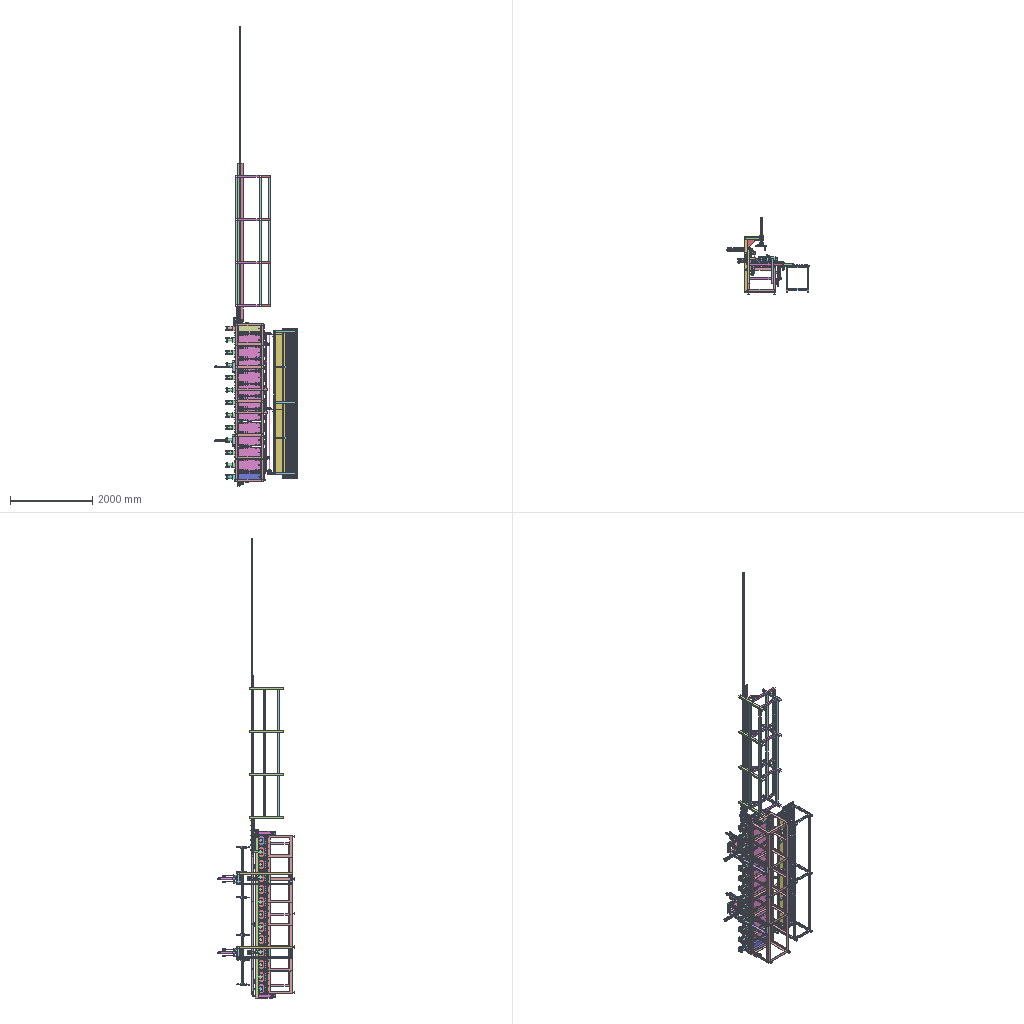Assembly | STEP file | 433 different items | 2728 placed | box 2000 x 1884 x 11210 mm
Parts list (item | name | quantity | parent item | size | volume), first 293 of 433 items:
1 | KHUNG SUON MAY DAP 3660 | x1 | in LAP KHUNG SUON MAY | 3868 x 784 x 600 mm | 15834108 mm3
2 | DIN 6915 M16 | x10 | in LAP KHUNG SUON MAY | 13 x 31.177 x 27 mm | 6064 mm3
3 | CHAN TANGDUA | x10 | in LAP KHUNG SUON MAY | 60 x 60 x 110 mm | 48381 mm3
4 | DIN 555 - replaced by DIN EN 24034 M16 | x8 | in LAP KHUNG SUON MAY | 13 x 27.713 x 24 mm | 4374 mm3
5 | DIN 6915 M12 | x52 | in LAP KHUNG SUON MAY | 10 x 25.403 x 22 mm | 3265 mm3
6 | MAT BAN CO LOGO 1_Welds | x1 | in MAT BAN CO LOGO 1 | 250 x 661.6 x 236 mm | 20450 mm3
7 | MAT BAN CO LOGO | x1 | in MAT BAN CO LOGO 1 | 250 x 633.6 x 80 mm | 6070480 mm3
8 | MAT TRUOT DAU BUA CO LOGO | x1 | in MAT BAN CO LOGO 1 | 250 x 300 x 24 mm | 1733556 mm3
9 | GA KHUON COI CO LOGO.dwg | x1 | in MAT BAN CO LOGO 1 | 250 x 186 x 260 mm | 3082669 mm3
10 | THANH CHINH NGAM TRUOT 2 | x2 | in MAT BAN CO LOGO 1 | 30 x 245 x 96 mm | 362252 mm3
11 | DAU BUA | x1 | in MAT BAN CO LOGO 1 | 130 x 95 x 200 mm | 1902985 mm3
12 | CHAN DO | x1 | in MAT BAN CO LOGO 1 | 250 x 55 x 70 mm | 565670 mm3
13 | CHAN DO2 | x1 | in MAT BAN CO LOGO 1 | 250 x 55 x 70 mm | 565670 mm3
14 | NGAM TRUOT | x1 | in MAT BAN CO LOGO 1 | 45 x 195 x 30 mm | 206561 mm3
15 | DIN 912 - replaced by DIN EN ISO 4762 M12 x 50 | x12 | in MAT BAN CO LOGO 1 | 62 x 18 x 18 mm | 8038 mm3
16 | DIN 912 - replaced by DIN EN ISO 4762 M14 x 40 | x9 | in MAT BAN CO LOGO 1 | 54 x 21 x 21 mm | 9880 mm3
17 | DIN 912 - replaced by DIN EN ISO 4762 M12 x 60 | x6 | in MAT BAN CO LOGO 1 | 72 x 18 x 18 mm | 9169 mm3
18 | DIN 912 - replaced by DIN EN ISO 4762 M10 x 50 | x6 | in MAT BAN CO LOGO 1 | 60 x 16 x 16 mm | 5580 mm3
19 | DIN 933 - replaced by DIN EN 24017 M10  x 40 | x4 | in MAT BAN CO LOGO 1 | 46.4 x 19.63 x 17 mm | 4638 mm3
20 | DIN 912 - replaced by DIN EN ISO 4762 M14 x 90 | x6 | in MAT BAN CO LOGO 1 | 104 x 21 x 21 mm | 17577 mm3
21 | MANG DAN PHOI CO LOGO | x1 | in MAT BAN CO LOGO 1 | 144 x 20 x 150 mm | 39222 mm3
22 | DIN 912 - replaced by DIN EN ISO 4762 M5 x 8 | x4 | in MAT BAN CO LOGO 1 | 13 x 8.5 x 8.5 mm | 395.808 mm3
23 | GA DAU NOI VAO DAU BUA | x1 | in MAT BAN CO LOGO 1 | 96 x 65 x 25 mm | 89450 mm3
24 | DAU NOI XY LANH 125 | x1 | in MAT BAN CO LOGO 1 | 56 x 56 x 39 mm | 36016 mm3
25 | Broached Socket Head Cap Screw - Metric M14x2 x 50 | x4 | in MAT BAN CO LOGO 1 | 64 x 21 x 21 mm | 11423 mm3
26 | giu lo xo day chot xien | x1 | in MAT BAN CO LOGO 1 | 80 x 25.5 x 50 mm | 77062 mm3
27 | Broached Socket Head Cap Screw - Metric M8x1.25 x 70 | x2 | in MAT BAN CO LOGO 1 | 78 x 13 x 13 mm | 4420 mm3
28 | Broached Hexagon Socket Set Screw - Flat Point - Metric M20x2.5 x 16 | x1 | in MAT BAN CO LOGO 1 | 16 x 20 x 20 mm | 3973 mm3
29 | Compress Spring1 | x1 | in Compress Spring | - | 1385 mm3
30 | TAM GA XYLANH GIUA | x1 | in MAT BAN CO LOGO 1 | 250 x 150 x 30 mm | 999493 mm3
31 | XYLANH _S_^80 | x1 | in MAT BAN CO LOGO 1 | 110 x 110 x 260 mm | 1251491 mm3
32 | PISTON XYLANH _S_^80 | x1 | in MAT BAN CO LOGO 1 | 40 x 40 x 118 mm | 134818 mm3
33 | TAN M35 BUOC 2 | x1 | in MAT BAN CO LOGO 1 | 57.735 x 50 x 14 mm | 16841 mm3
34 | NGAM TRUOT 2 | x1 | in MAT BAN CO LOGO 1 | 45 x 195 x 30 mm | 206561 mm3
35 | CHOT 14X100 | x4 | in MAT BAN CO LOGO 1 | 14 x 14 x 100 mm | 15235 mm3
36 | MIENG TRUNG GIAN DUOI | x1 | in KHUON AM CO LOGO | 250 x 135 x 24 mm | 656672 mm3
37 | KHUON BAO DUOI | x1 | in KHUON AM CO LOGO | 135 x 250 x 39.2 mm | 803564 mm3
38 | CHOT DINH VI 40 | x2 | in KHUON AM CO LOGO | 8 x 8 x 60 mm | 2993 mm3
39 | KHUON AM | x1 | in KHUON AM CO LOGO | 122.5 x 70 x 45.5 mm | 234393 mm3
40 | LOGO LOI | x1 | in KHUON AM CO LOGO | 22 x 16.4 x 40.3 mm | 10596 mm3
41 | LUOI GA TRON DUOI | x1 | in KHUON AM CO LOGO | 17 x 7 x 40.799 mm | 3679 mm3
42 | AS 1420 - Metric M8 x 25 | x6 | in KHUON AM CO LOGO | 33 x 13 x 13 mm | 2157 mm3
43 | AS 1420 - Metric M10 x 45 | x6 | in KHUON AM CO LOGO | 55 x 16 x 16 mm | 5187 mm3
44 | dao nhan khuon dap 3m6 | x1 | in KHUON AM CO LOGO | 45 x 34.3 x 57.1 mm | 58767 mm3
45 | con truot | x1 | in KHUON AM CO LOGO | 76 x 17 x 12 mm | 11883 mm3
46 | chot xien con truot | x1 | in KHUON AM CO LOGO | 15 x 47.7 x 30 mm | 18730 mm3
47 | cu dao nhan | x1 | in KHUON AM CO LOGO | 100 x 63 x 20 mm | 110399 mm3
48 | con chan chot xien | x1 | in KHUON AM CO LOGO | 20 x 10 x 18 mm | 1960 mm3
49 | Broached Socket Head Cap Screw - Metric M10x1.5 x 35 | x2 | in KHUON AM CO LOGO | 45 x 16 x 16 mm | 4403 mm3
50 | Broached Socket Head Cap Screw - Metric M10x1.5 x 50 | x1 | in KHUON AM CO LOGO | 60 x 16 x 16 mm | 5581 mm3
51 | Broached Socket Head Cap Screw - Metric M10x1.5 x 40 | x5 | in KHUON AM CO LOGO | 50 x 16 x 16 mm | 4795 mm3
52 | Broached Socket Head Cap Screw - Metric M6x1 x 16 | x1 | in KHUON AM CO LOGO | 22 x 10 x 10 mm | 839.144 mm3
53 | Broached Socket Head Cap Screw - Metric M10x1.5 x 30 | x1 | in KHUON AM CO LOGO | 40 x 16 x 16 mm | 4010 mm3
54 | luoi ga co logo | x1 | in KHUON AM CO LOGO | 10 x 15.6 x 51.124 mm | 6311 mm3
55 | Compress Spring1_2 | x1 | in Compress Spring_2 | - | 492.963 mm3
56 | Broached Socket Head Cap Screw - Metric M5x0.8 x 25 | x1 | in KHUON AM CO LOGO | 30 x 8.5 x 8.5 mm | 729.698 mm3
57 | BAT VOI MANG CA CO LOGO | x1 | in KHUON DUONG CO LOGO | 250 x 135 x 24 mm | 764464 mm3
58 | MIENG DE KHUON DUONG CO LOGO | x1 | in KHUON DUONG CO LOGO | 250 x 135 x 24 mm | 741333 mm3
59 | KHUON BAO TREN | x1 | in KHUON DUONG CO LOGO | 135 x 250 x 53 mm | 1111090 mm3
60 | CHOT DINH VI | x2 | in KHUON DUONG CO LOGO | 8 x 8 x 75 mm | 3747 mm3
61 | KHUON DUONG | x1 | in KHUON DUONG CO LOGO | 122.5 x 70 x 55.2 mm | 288291 mm3
62 | LUOI CAT | x1 | in KHUON DUONG CO LOGO | 88.8 x 70 x 40 mm | 196550 mm3
63 | LOGO LOM | x1 | in KHUON DUONG CO LOGO | 22 x 16.4 x 54.3 mm | 14617 mm3
64 | LUOI GA PHIA TREN | x1 | in KHUON DUONG CO LOGO | 17.5 x 11 x 53.3 mm | 9330 mm3
65 | LUOI GA TRON PHIA TREN | x1 | in KHUON DUONG CO LOGO | 17 x 7 x 57.44 mm | 5792 mm3
66 | THAN GA LUOI DOT | x1 | in KHUON DUONG CO LOGO | 14 x 22.5 x 77 mm | 19378 mm3
67 | LUOI DOT | x1 | in KHUON DUONG CO LOGO | 4 x 15.5 x 65.8 mm | 3850 mm3
68 | CHOT DUC 6.0 | x2 | in KHUON DUONG CO LOGO | 80 x 12.5 x 12.5 mm | 6322 mm3
69 | CHOT CAI | x1 | in KHUON DUONG CO LOGO | 6 x 6 x 22 mm | 620.89 mm3
70 | AS 1420 - Metric M8 x 30 | x1 | in KHUON DUONG CO LOGO | 38 x 13 x 13 mm | 2408 mm3
71 | AS 1420 - Metric M5 x 30 | x2 | in KHUON DUONG CO LOGO | 35 x 8.5 x 8.5 mm | 827.769 mm3
72 | AS 1420 - Metric M10 x 45_2 | x5 | in KHUON DUONG CO LOGO | 95 x 16 x 16 mm | 8328 mm3
73 | AS 1420 - Metric M8 x 55 | x1 | in KHUON DUONG CO LOGO | 63 x 13 x 13 mm | 3665 mm3
74 | CHOT TRUOT 6 LY | x4 | in KHUON DUONG CO LOGO | 6 x 6 x 8 mm | 225.049 mm3
75 | chot cam | x1 | in KHUON DUONG CO LOGO | 30 x 15 x 95 mm | 41659 mm3
76 | Broached Socket Head Cap Screw - Metric M10x1.5 x 80 | x5 | in KHUON DUONG CO LOGO | 90 x 16 x 16 mm | 7937 mm3
77 | Broached Socket Head Cap Screw - Metric M8x1.25 x 60 | x1 | in KHUON DUONG CO LOGO | 68 x 13 x 13 mm | 3917 mm3
78 | CHOT DAN DUONG | x4 | in KHUON DUONG CO LOGO | 18 x 18 x 95 mm | 15092 mm3
79 | Broached Socket Head Cap Screw - Metric M8x1.25 x 30 | x4 | in KHUON DUONG CO LOGO | 38 x 13 x 13 mm | 2409 mm3
80 | Broached Socket Head Cap Screw - Metric M5x0.8 x 25_2 | x2 | in KHUON DUONG CO LOGO | 30 x 8.5 x 8.5 mm | 729.698 mm3
81 | Broached Socket Head Cap Screw - Metric M12x1.75 x 30 | x4 | in KHUON DUONG CO LOGO | 42 x 18 x 18 mm | 5780 mm3
82 | noi khi | x1 | in KHUON DUONG CO LOGO | 37 x 27 x 14 mm | 4436 mm3
83 | MAT BAN KHONG LOGO_Welds | x1 | in 84 | 250 x 661.6 x 236 mm | 20450 mm3
84 | MAT BAN KHONG LOGO | x1 | in 84 | 250 x 633.6 x 80 mm | 6062488 mm3
85 | MAT TRUOT DAU BUA KHONG LOGO | x1 | in 84 | 250 x 300 x 24 mm | 1737062 mm3
86 | GA KHUON COI KHONG LOGO | x1 | in 84 | 250 x 186 x 203 mm | 2822642 mm3
87 | NGAM TRUOT_2 | x1 | in 84 | 45 x 195 x 30 mm | 206561 mm3
88 | THANH CHINH NGAM TRUOT 2_2 | x2 | in 84 | 30 x 245 x 96 mm | 362252 mm3
89 | CHAN DO_2 | x1 | in 84 | 250 x 55 x 70 mm | 565670 mm3
90 | DAU BUA_2 | x1 | in 84 | 130 x 95 x 200 mm | 1902822 mm3
91 | CHAN DO2_2 | x1 | in 84 | 250 x 55 x 70 mm | 565670 mm3
92 | DIN 912 - replaced by DIN EN ISO 4762 M14 x 35 | x7 | in 84 | 49 x 21 x 21 mm | 9111 mm3
93 | DIN 912 - replaced by DIN EN ISO 4762 M12 x 50_2 | x10 | in 84 | 62 x 18 x 18 mm | 8038 mm3
94 | DIN 912 - replaced by DIN EN ISO 4762 M14 x 50 | x4 | in 84 | 64 x 21 x 21 mm | 11420 mm3
95 | DIN 912 - replaced by DIN EN ISO 4762 M10 x 50_2 | x6 | in 84 | 60 x 16 x 16 mm | 5580 mm3
96 | DIN 933 - replaced by DIN EN 24017 M10  x 40_2 | x4 | in 84 | 46.4 x 19.63 x 17 mm | 4638 mm3
97 | DIN 912 - replaced by DIN EN ISO 4762 M10 x 40 | x4 | in 84 | 50 x 16 x 16 mm | 4794 mm3
98 | DIN 912 - replaced by DIN EN ISO 4762 M12 x 60_2 | x4 | in 84 | 72 x 18 x 18 mm | 9169 mm3
99 | DIN 912 - replaced by DIN EN ISO 4762 M12 x 70 | x4 | in 84 | 82 x 18 x 18 mm | 10300 mm3
100 | DIN 912 - replaced by DIN EN ISO 4762 M14 x 40_2 | x2 | in 84 | 54 x 21 x 21 mm | 9880 mm3
101 | DIN 912 - replaced by DIN EN ISO 4762 M14 x 90_2 | x6 | in 84 | 104 x 21 x 21 mm | 17577 mm3
102 | MANG DAN PHOI KHONG LOGO | x1 | in 84 | 144 x 20 x 150 mm | 39222 mm3
103 | DIN 912 - replaced by DIN EN ISO 4762 M5 x 8_2 | x4 | in 84 | 13 x 8.5 x 8.5 mm | 395.808 mm3
104 | CHOT 14X100_2 | x4 | in 84 | 14 x 14 x 100 mm | 15235 mm3
105 | NGAM TRUOT 2_2 | x1 | in 84 | 45 x 195 x 30 mm | 206561 mm3
106 | GA DAU NOI VAO DAU BUA_2 | x1 | in 84 | 96 x 65 x 25 mm | 89450 mm3
107 | PISTON XYLANH _S_^80_2 | x1 | in 84 | 40 x 40 x 118 mm | 134818 mm3
108 | XYLANH _S_^80_2 | x1 | in 84 | 110 x 110 x 260 mm | 1251491 mm3
109 | TAM GA XYLANH GIUA_2 | x1 | in 84 | 250 x 150 x 30 mm | 999493 mm3
110 | DAU NOI XY LANH 80 2 DAU NGAM | x1 | in 84 | 56 x 56 x 39 mm | 36016 mm3
111 | MIENG DE KHUON AM KO LOGO | x1 | in KHUON AM KHONG LOGO | 250 x 135 x 24 mm | 675291 mm3
112 | KHUON BAO DUOI_2 | x1 | in KHUON AM KHONG LOGO | 135 x 250 x 39.2 mm | 811850 mm3
113 | KHUON AM_2 | x1 | in KHUON AM KHONG LOGO | 122.5 x 70 x 45.5 mm | 246860 mm3
114 | LUOI GA PHIA DUOI | x1 | in KHUON AM KHONG LOGO | 17.5 x 11 x 39 mm | 7111 mm3
115 | LUOI GA TRON PHIA DUOI | x1 | in KHUON AM KHONG LOGO | 17 x 7 x 42.5 mm | 4171 mm3
116 | AS 1420 - Metric M5 x 30_2 | x2 | in KHUON AM KHONG LOGO | 35 x 8.5 x 8.5 mm | 827.769 mm3
117 | AS 1420 - Metric M8 x 25_2 | x3 | in KHUON AM KHONG LOGO | 33 x 13 x 13 mm | 2157 mm3
118 | AS 1420 - Metric M10 x 50 | x5 | in KHUON AM KHONG LOGO | 60 x 16 x 16 mm | 5580 mm3
119 | CHOT DINH VI 40_2 | x2 | in KHUON AM KHONG LOGO | 8 x 8 x 60 mm | 2993 mm3
120 | cu dao nhan khong logo | x1 | in KHUON AM KHONG LOGO | 110 x 63 x 20 mm | 127794 mm3
121 | Broached Socket Head Cap Screw - Metric M10x1.5 x 50_2 | x5 | in KHUON AM KHONG LOGO | 60 x 16 x 16 mm | 5581 mm3
122 | Broached Socket Head Cap Screw - Metric M10x1.5 x 40_2 | x1 | in KHUON AM KHONG LOGO | 50 x 16 x 16 mm | 4795 mm3
123 | Broached Socket Head Cap Screw - Metric M10x1.5 x 30_2 | x1 | in KHUON AM KHONG LOGO | 40 x 16 x 16 mm | 4010 mm3
124 | Broached Socket Head Cap Screw - Metric M8x1.25 x 30_2 | x4 | in KHUON AM KHONG LOGO | 38 x 13 x 13 mm | 2409 mm3
125 | Broached Socket Head Cap Screw - Metric M5x0.8 x 25_3 | x2 | in KHUON AM KHONG LOGO | 30 x 8.5 x 8.5 mm | 729.698 mm3
126 | Broached Socket Head Cap Screw - Metric M8x1.25 x 40 | x1 | in KHUON AM KHONG LOGO | 48 x 13 x 13 mm | 2912 mm3
127 | Broached Socket Head Cap Screw - Metric M10x1.5 x 35_2 | x2 | in KHUON AM KHONG LOGO | 45 x 16 x 16 mm | 4403 mm3
128 | Compress Spring1_3 | x1 | in Compress Spring_3 | - | 492.963 mm3
129 | dao nhan khong logo | x1 | in KHUON AM KHONG LOGO | 38 x 36 x 57.1 mm | 51330 mm3
130 | BAT VOI MANG CA KO LOGO | x1 | in KHUON DUONG KHONG LOGO | 250 x 135 x 24 mm | 764621 mm3
131 | MIENG DE KHUON DUONG KO LOGO | x1 | in KHUON DUONG KHONG LOGO | 250 x 135 x 24 mm | 743044 mm3
132 | EES - 2C 12x100 | x1 | in KHUON DUONG KHONG LOGO | 18 x 18 x 80 mm | 12722 mm3
133 | KHUON BAO TREN_2 | x1 | in KHUON DUONG KHONG LOGO | 135 x 250 x 53 mm | 1110961 mm3
134 | CHOT DINH VI_2 | x2 | in KHUON DUONG KHONG LOGO | 8 x 8 x 70 mm | 3496 mm3
135 | KHUON DUONG_2 | x1 | in KHUON DUONG KHONG LOGO | 122.5 x 70 x 55 mm | 306755 mm3
136 | LUOI CAT KHONG LOGO | x1 | in KHUON DUONG KHONG LOGO | 88.8 x 70 x 40 mm | 196221 mm3
137 | LUOI GA PHAI TREN | x1 | in KHUON DUONG KHONG LOGO | 10 x 15.6 x 59.05 mm | 8567 mm3
138 | LUOI GA TRON TREN | x1 | in KHUON DUONG KHONG LOGO | 17 x 7 x 55.799 mm | 5306 mm3
139 | CHOT CAI_2 | x1 | in KHUON DUONG KHONG LOGO | 6 x 6 x 22 mm | 620.89 mm3
140 | CHOT DUC 6.0_2 | x2 | in KHUON DUONG KHONG LOGO | 80 x 12.5 x 12.5 mm | 6322 mm3
141 | LUOI DOT_2 | x1 | in KHUON DUONG KHONG LOGO | 4 x 15.5 x 65.8 mm | 3850 mm3
142 | THAN GA LUOI DOT_2 | x1 | in KHUON DUONG KHONG LOGO | 14 x 22.5 x 77 mm | 19378 mm3
143 | AS 1420 - Metric M8 x 30_2 | x3 | in KHUON DUONG KHONG LOGO | 68 x 13 x 13 mm | 3916 mm3
144 | AS 1420 - Metric M5 x 30_3 | x2 | in KHUON DUONG KHONG LOGO | 35 x 8.5 x 8.5 mm | 827.769 mm3
145 | EES - 2C 12x100_2 | x3 | in KHUON DUONG KHONG LOGO | 18 x 18 x 100 mm | 15801 mm3
146 | AS 1420 - Metric M10 x 45_3 | x1 | in KHUON DUONG KHONG LOGO | 95 x 16 x 16 mm | 8328 mm3
147 | Compress Spring1_4 | x1 | in Compress Spring_4 | - | 3363 mm3
148 | CHOT TRUOT 6 LY_2 | x4 | in KHUON DUONG KHONG LOGO | 6 x 6 x 8 mm | 225.049 mm3
149 | chot cam_2 | x1 | in KHUON DUONG KHONG LOGO | 30 x 15 x 95 mm | 41659 mm3
150 | Broached Socket Head Cap Screw - Metric M8x1.25 x 30_3 | x1 | in KHUON DUONG KHONG LOGO | 38 x 13 x 13 mm | 2409 mm3
151 | Broached Socket Head Cap Screw - Metric M10x1.5 x 80_2 | x5 | in KHUON DUONG KHONG LOGO | 90 x 16 x 16 mm | 7937 mm3
152 | noi khi_2 | x1 | in KHUON DUONG KHONG LOGO | 37 x 27 x 14 mm | 4436 mm3
153 | MAT BAN GIUA_Welds | x11 | in 154 | 270 x 661.6 x 216 mm | 46200 mm3
154 | MAT BAN GIUA | x11 | in 154 | 270 x 633.6 x 80 mm | 5694476 mm3
155 | TAM TRUOT DAU BUA GIUA | x11 | in 154 | 270 x 300 x 24 mm | 1881062 mm3
156 | GA KHUON COI GIUA.dwg | x11 | in 154 | 270 x 166 x 203 mm | 2828600 mm3
157 | NGAM TRUOT_3 | x11 | in 154 | 45 x 194 x 30 mm | 205453 mm3
158 | THANH CHINH NGAM TRUOT 2_3 | x22 | in 154 | 30 x 294 x 96 mm | 428402 mm3
159 | DAU BUA_3 | x11 | in 154 | 130 x 95 x 200 mm | 1901919 mm3
160 | DIN 912 - replaced by DIN EN ISO 4762 M10 x 50_3 | x66 | in 154 | 60 x 16 x 16 mm | 5580 mm3
161 | DIN 912 - replaced by DIN EN ISO 4762 M14 x 35_2 | x99 | in 154 | 49 x 21 x 21 mm | 9111 mm3
162 | CHAN DO MAT BAN GIUA | x11 | in 154 | 270 x 55 x 70 mm | 612670 mm3
163 | CHAN DO MAT BAN GIUA BEN COI | x11 | in 154 | 270 x 55 x 70 mm | 612670 mm3
164 | DIN 912 - replaced by DIN EN ISO 4762 M12 x 50_3 | x110 | in 154 | 62 x 18 x 18 mm | 8038 mm3
165 | DIN 912 - replaced by DIN EN ISO 4762 M12 x 60_3 | x44 | in 154 | 72 x 18 x 18 mm | 9169 mm3
166 | DIN 912 - replaced by DIN EN ISO 4762 M12 x 70_2 | x44 | in 154 | 82 x 18 x 18 mm | 10300 mm3
167 | DIN 960 - replaced by DIN EN 28765 M10 x 1.25 x 40 | x44 | in 154 | 46.4 x 19.63 x 17 mm | 4694 mm3
168 | DIN 912 - replaced by DIN EN ISO 4762 M14 x 90_3 | x66 | in 154 | 104 x 21 x 21 mm | 17577 mm3
169 | MANG DAN PHOI BO GIUA | x11 | in 154 | 164 x 20 x 150 mm | 43722 mm3
170 | DIN 912 - replaced by DIN EN ISO 4762 M5 x 8_3 | x44 | in 154 | 13 x 8.5 x 8.5 mm | 395.808 mm3
171 | XYLANH _S_^80_3 | x11 | in 154 | 110 x 110 x 260 mm | 1251491 mm3
172 | TAM GA XYLANH GIUA_3 | x11 | in 154 | 250 x 150 x 30 mm | 1040750 mm3
173 | PISTON XYLANH _S_^80_3 | x11 | in 154 | 40 x 40 x 118 mm | 134818 mm3
174 | TAN M35 BUOC 2_2 | x11 | in 154 | 57.735 x 50 x 14 mm | 16841 mm3
175 | GA DAU NOI VAO DAU BUA_3 | x11 | in 154 | 96 x 65 x 25 mm | 89450 mm3
176 | DAU NOI BUA GIUA | x11 | in 154 | 76.5 x 56 x 56 mm | 107628 mm3
177 | BAC XAC DINH VI TRI XYLANH 80 | x11 | in 154 | 55 x 55 x 4 mm | 5655 mm3
178 | Broached Socket Head Cap Screw - Metric M14x2 x 50_2 | x44 | in 154 | 64 x 21 x 21 mm | 11423 mm3
179 | Broached Socket Head Cap Screw - Metric M10x1.5 x 45 | x44 | in 154 | 55 x 16 x 16 mm | 5188 mm3
180 | NGAM TRUOT 2_3 | x11 | in 154 | 45 x 194 x 30 mm | 205453 mm3
181 | CHOT 14X100_3 | x44 | in 154 | 14 x 14 x 100 mm | 15235 mm3
182 | TAM DE COI | x11 | in KHUON AM GIUA | 270 x 100 x 39 mm | 987341 mm3
183 | TAM COI | x11 | in KHUON AM GIUA | 270 x 68 x 25 mm | 392735 mm3
184 | DIN EN 22338 A - withdrawn 8 m6 x 40 - A | x22 | in KHUON AM GIUA | 40 x 8 x 8 mm | 1978 mm3
185 | DIN 912 - replaced by DIN EN ISO 4762 M8 x 50 | x66 | in KHUON AM GIUA | 58 x 13 x 13 mm | 3414 mm3
186 | TAM DE CHAY | x11 | in KHUON DUONG GIUA | 270 x 100 x 30 mm | 752474 mm3
187 | TAM LOT CHAY | x11 | in KHUON DUONG GIUA | 270 x 100 x 15 mm | 381434 mm3
188 | TAM GA CHAY | x11 | in KHUON DUONG GIUA | 270 x 100 x 30 mm | 706425 mm3
189 | COT DAN HUONG14X73 | x22 | in KHUON DUONG GIUA | 18 x 18 x 73 mm | 11705 mm3
190 | CHAY 6X10X50.dwg | x44 | in KHUON DUONG GIUA | 50 x 13 x 13 mm | 3399 mm3
191 | TAM CHAN PHOI | x11 | in KHUON DUONG GIUA | 270 x 24 x 12 mm | 71324 mm3
192 | DIN 912 - replaced by DIN EN ISO 4762 M12 x 40 | x44 | in KHUON DUONG GIUA | 52 x 18 x 18 mm | 6908 mm3
193 | DIN 912 - replaced by DIN EN ISO 4762 M8 x 30 | x44 | in KHUON DUONG GIUA | 38 x 13 x 13 mm | 2408 mm3
194 | DIN 912 - replaced by DIN EN ISO 4762 M8 x 60 | x66 | in KHUON DUONG GIUA | 68 x 13 x 13 mm | 3916 mm3
195 | BULONG BAC M8X10X56 | x22 | in KHUON DUONG GIUA | 15 x 15 x 74 mm | 6196 mm3
196 | bac 10.5-28 | x22 | in KHUON DUONG GIUA | 28 x 28 x 8 mm | 4233 mm3
197 | CU AN TOAN 10.4-20 - 5.5 | x22 | in KHUON DUONG GIUA | 30 x 30 x 5.5 mm | 1797 mm3
198 | LO XO D20d3X36 | x22 | in KHUON DUONG GIUA | 20.006 x 39.001 x 20.006 mm | 2345 mm3
199 | BULONG BAC M8X10X38 | x22 | in KHUON DUONG GIUA | 15 x 15 x 58 mm | 4939 mm3
200 | Compress Spring1_5 | x22 | in Compress Spring_5 | - | 1934 mm3
201 | CHAY 3.9 | x22 | in KHUON DUONG GIUA | 4 x 15.5 x 50 mm | 2874 mm3
202 | CHOT DINH VI 4X10 | x22 | in KHUON DUONG GIUA | 4 x 4 x 10 mm | 120.876 mm3
203 | Thanh T chinh 3m6 | x11 | in Automatic feeder punching | 24 x 37.5 x 3660 mm | 442294 mm3
204 | BCC3 H11_1B | x1 | in BCC3 H11B | 60 x 60 x 3440 mm | 1915667 mm3
205 | BCC3 H11_2B | x3 | in BCC3 H11B | 80 x 40 x 45 mm | 55899 mm3
206 | BCC3 H11_3 | x8 | in BCC3 H11B, BCC3 H12B, BCC3 H11_2 | 20 x 20 x 50 mm | 15708 mm3
207 | BCC3 H12_7B | x1 | in 207 | 40 x 75 x 4068 mm | 2791952 mm3
208 | BCC3 H12_8B | x2 | in 207 | 40 x 100 x 340 mm | 276708 mm3
209 | BCC3 H12_13 | x2 | in 207 | 70 x 68 x 10 mm | 46465 mm3
210 | Bulong M10_2.5F | x39 | in BCC3 G02B Motion1, BCC3 G03B Motion1, Automatic feeder punching | 18.475 x 16 x 31.5 mm | 3390 mm3
211 | Tan M10 | x23 | in BCC3 G02B Motion1, Automatic feeder punching, 237 | 18.475 x 16 x 9 mm | 1288 mm3
212 | BCC3 H11_5 | x10 | in BCC3 G02B Motion1, 237 | 15 x 15 x 1 mm | 90.124 mm3
213 | 6800ZZ | x7 | in BCC3 G02B Motion1 | 19 x 19 x 5 mm | 1015 mm3
214 | BCC3 H11_4 | x10 | in BCC3 G02B Motion1, 237 | 14 x 14 x 27 mm | 2265 mm3
215 | BCC3 H13_1 | x2 | in BCC3 G03B Motion1 | 290 x 22 x 100 mm | 496185 mm3
216 | - | x2 | - | 491 x 50.3 x 52 mm | 426363 mm3
217 | - | x6 | in BCC3 G03B Motion1, BCC3 G03B Motion2 | 471 x 40 x 40 mm | 111313 mm3
218 | 201100_M42x1_5_HI | x2 | - | 53.666 x 53.666 x 12 mm | 11002 mm3
219 | Bac truot | x4 | in BCC3 G03B Motion1 | 60 x 60 x 80 mm | 114067 mm3
220 | BCC3 H13_8B | x2 | in BCC3 H13_6B | 40 x 75 x 475 mm | 326568 mm3
221 | BCC3 H13_8B | x2 | in BCC3 H13_6B | 40 x 75 x 475 mm | 326568 mm3
222 | BCC3 H13_7 | x4 | in BCC3 H13_6B | 40 x 75 x 210 mm | 145356 mm3
223 | BCC3 H13_6 | x2 | in BCC3 H13_6B | 40 x 75 x 1270 mm | 877986 mm3
224 | BCC3 H13_6 | x2 | in BCC3 H13_6B | 40 x 75 x 1270 mm | 877986 mm3
225 | BCC3 H13_7 | x2 | in BCC3 H13_6B | 40 x 75 x 210 mm | 144819 mm3
226 | BCC3 H13_9B | x4 | in BCC3 H13_6B | 200 x 200 x 6 mm | 120000 mm3
227 | BCC3 H13_7 | x2 | in BCC3 H13_6B | 40 x 75 x 210 mm | 144819 mm3
228 | BCC3 H13_10 | x4 | in BCC3 H13_6B | 40 x 75 x 6 mm | 16643 mm3
229 | BCC3 H14_3B | x2 | in BCC3 H14B2_HI | 57 x 274 x 60 mm | 86752 mm3
230 | BCC3 H14_6B | x8 | in BCC3 H14B2_HI | 45 x 100 x 6 mm | 13452 mm3
231 | BCC3 H14_7 | x2 | in BCC3 H14B2_HI | 40 x 40 x 120 mm | 112909 mm3
232 | - | x2 | - | 50 x 50 x 517 mm | 322395 mm3
233 | - | x4 | in Automatic feeder punching | 32 x 32 x 503.2 mm | 60225 mm3
234 | - | x8 | in BCC3 G05 Motion1, Automatic feeder punching | 17 x 5 x 19.63 mm | 939.625 mm3
235 | BCC3 H16_1 | x3 | in 235 | 500 x 80 x 6 mm | 213344 mm3
236 | BCC3 H16_4 | x3 | in 235 | 32 x 16 x 32 mm | 8049 mm3
237 | BCC3 H16_7 | x3 | in 235 | 55 x 55 x 40 mm | 65270 mm3
238 | BCC3 H16_15 | x3 | in 235 | 20 x 20 x 230 mm | 17480 mm3
239 | BCC3 H16_5 | x3 | in BCC3 G05_1 | 25 x 25 x 8 mm | 1414 mm3
240 | BCC3 H16_2 | x3 | in BCC3 G05_1 | 95 x 10 x 95 mm | 53732 mm3
241 | BCC3 H16_6 | x3 | in BCC3 G05_1 | 30 x 30 x 2 mm | 1313 mm3
242 | Bulong M6_1.5F | x7 | in BCC3 G05_1, BCC3 G03B Motion2 | 11.547 x 10 x 19 mm | 768.3 mm3
243 | BCC3 H16_3 | x3 | in BCC3 G05_1 | 95 x 30 x 95 mm | 74080 mm3
244 | BCC3 H16_9 | x3 | in BCC3 G05_1 | 55 x 55 x 12 mm | 13803 mm3
245 | BCC3 H16_10 | x3 | in BCC3 G05_1 | 499.144 x 99.144 x 8 mm | 58375 mm3
246 | Bulong M8_2.5F | x6 | in BCC3 G05_1 | 12.73 x 14.699 x 30.15 mm | 1976 mm3
247 | BCC3 H16_8 | x1 | in BCC3 G05_2 | 25 x 25 x 3385 mm | 2110006 mm3
248 | BCC3 H16_11 | x4 | in BCC3 G05 Motion1, BCC3 H14B1_HI | 20 x 550 x 20 mm | 172727 mm3
249 | BCC3 H16_12 | x2 | in BCC3 G05 Motion1 | 83 x 40 x 30 mm | 84627 mm3
250 | BCC3 H16_13 | x1 | in BCC3 G05 Motion1 | 20 x 20 x 3390 mm | 1063554 mm3
251 | Gear motor - 12V (6 holes)_Default | x1 | in BCC3 G05 Motion1 | 124.05 x 100.1 x 199.5 mm | 340663 mm3
252 | BCC3 H16_14 | x1 | in BCC3 G05 Motion1 | 120 x 80 x 15 mm | 111656 mm3
253 | BCC3 H16_16 | x3 | in BCC3 G05 Motion1 | 5 x 5 x 30 mm | 750 mm3
254 | Bulong M8_2F | x8 | in BCC3 G05 Motion1, Automatic feeder punching | 12.73 x 14.699 x 25.15 mm | 1725 mm3
255 | - | x4 | in BCC3 G05 Motion1 | 32 x 32 x 303.2 mm | 37606 mm3
256 | BCC3 H17_1 | x2 | in BCC3 H17_HI | 130 x 120 x 60 mm | 136586 mm3
257 | BCC3 H17_2 | x2 | in BCC3 H17_HI | 40 x 40 x 150 mm | 141183 mm3
258 | BCC3 H17_3 | x4 | in BCC3 H17_HI | 120 x 90 x 6 mm | 32400 mm3
259 | - | x2 | - | 50 x 50 x 317 mm | 245584 mm3
260 | BCC3 H12_1B | x1 | in BCC3 H12B | 60 x 60 x 3968 mm | 2197436 mm3
261 | BCC3 H12_2B | x2 | in BCC3 H12B | 65 x 40 x 10 mm | 23230 mm3
262 | BCC3 H12_10 | x4 | in 262 | 75 x 30 x 18 mm | 28180 mm3
263 | 6300ZZ | x7 | in 262, 237 | 35 x 35 x 11 mm | 9704 mm3
264 | BCC3 H12_11 | x4 | in 262 | 12 x 32 x 12 mm | 2579 mm3
265 | BCC3 H12_12 | x4 | in 262 | 16 x 3 x 16 mm | 358.047 mm3
266 | countersunk flat head cross recess screw_din_ISO 7046-1 - M5 x 8 - Z --- 8N | x8 | in BCC3 H12B | 8 x 9.3 x 9.3 mm | 212.099 mm3
267 | BCC3 H12_5 | x2 | in Automatic feeder punching | 48 x 55 x 90 mm | 65386 mm3
268 | - | x2 | - | 50 x 50 x 242 mm | 216779 mm3
269 | - | x4 | in Automatic feeder punching | 32 x 32 x 228.2 mm | 29124 mm3
270 | Do phoi 11 | x2 | - | 50 x 55 x 50 mm | 41866 mm3
271 | BCC3 H12_4B | x2 | in Automatic feeder punching | 30 x 64 x 20 mm | 31837 mm3
272 | Bulong M16_4F | x4 | in Automatic feeder punching | 27.713 x 24 x 50 mm | 13007 mm3
273 | BCC3 H13_2 | x2 | in BCC3 H13 | 200 x 90 x 55 mm | 586969 mm3
274 | BCC3 H13_3 | x4 | in BCC3 H13 | 25 x 400 x 25 mm | 195748 mm3
275 | Lo xo bac truot | x8 | in BCC3 H13 | 32 x 62 x 32 mm | 1777 mm3
276 | BCC3 H13_4 | x4 | in BCC3 H13 | 35 x 3 x 35 mm | 2771 mm3
277 | BCC3 H13_5 | x1 | in BCC3 G03B Motion2 | 45 x 45 x 3395 mm | 4368342 mm3
278 | LG M8_3F | x12 | in BCC3 G03B Motion2 | 14 x 14 x 38 mm | 2614 mm3
279 | BCC3 H13_11 | x6 | in BCC3 G03B Motion2 | 70 x 50 x 50 mm | 62756 mm3
280 | LG M6_2F | x66 | in BCC3 G03B Motion2, Ngam kep Motion1, Ngam kep Motion2 | 10 x 10 x 26 mm | 971.253 mm3
281 | 9123_DGS_16_10_P_z_HI | x6 | - | 142 x 27 x 27 mm | 38230 mm3
282 | 9123_DGS_16_10_P_k_HI | x6 | - | 111 x 16 x 16 mm | 6739 mm3
283 | Tan M8 | x13 | in Automatic feeder punching | 12.73 x 14.699 x 7 mm | 737.742 mm3
284 | LG M6_1.5F | x36 | in BCC3 G03B Motion2, Bo cuon T phu | 10 x 10 x 21 mm | 829.881 mm3
285 | 4935_DGS_16_1_P_z_HI | x6 | - | 115 x 27 x 27 mm | 36319 mm3
286 | 4935_DGS_16_1_P_k_HI | x12 | in Automatic feeder punching | 102 x 16 x 16 mm | 6287 mm3
287 | 204596_DIN176_M20x1_5_7_24_HI | x6 | - | 6 x 31.177 x 27 mm | 2144 mm3
288 | Ngam kep 7 | x6 | in Ngam kep Motion1 | 100 x 70 x 60 mm | 42428 mm3
289 | Ngam kep 9 | x6 | in Ngam kep Motion1 | 90 x 15 x 60 mm | 65238 mm3
290 | Ngam kep 8 | x6 | in Ngam kep Motion1 | 15 x 15 x 27 mm | 3046 mm3
291 | Ngam kep 19 | x6 | in Ngam kep Motion1 | 13 x 44 x 13 mm | 652.249 mm3
292 | plain washer 10669 type nl_iso_PreviewCfg | x6 | in Ngam kep Motion1 | 2 x 20 x 20 mm | 506.676 mm3
293 | Ngam kep 1 | x6 | in Ngam kep Motion2 | 135 x 70 x 24 mm | 65929 mm3
Placements (level | parent | child | x y z in mm | rotation matrix by rows), first 171 of 2915 lines:
1 | Automatic feeder punching | LAP HOAN CHINH | -670.0 -0.0 -3868.0 | 0 1 0 0 0 1 1 0 -0
2 | LAP HOAN CHINH | KHUNG DO KHUON DAP 3660 | -0.0 -0.0 -0.0 | 1 0 0 0 1 0 0 0 1
3 | KHUNG DO KHUON DAP 3660 | LAP KHUNG SUON MAY | -0.0 -0.0 -0.0 | 1 0 0 0 1 0 0 0 1
4 | LAP KHUNG SUON MAY | KHUNG SUON MAY DAP 3660 | -0.0 -0.0 -0.0 | 1 0 0 0 1 0 0 0 1
4 | LAP KHUNG SUON MAY | DIN 6915 M16 | 2800.0 6.0 17.0 | 0 0 1 0 1 0 -1 0 -0
4 | LAP KHUNG SUON MAY | DIN 6915 M16 | 2800.0 6.0 -13.0 | 0 0 -1 0 1 0 1 0 0
4 | LAP KHUNG SUON MAY | CHAN TANGDUA | 2800.0 6.0 -60.0 | 1 0 0 0 1 0 0 0 1
4 | LAP KHUNG SUON MAY | CHAN TANGDUA | 2800.0 640.0 -60.0 | 1 0 0 0 1 0 0 0 1
4 | LAP KHUNG SUON MAY | DIN 555 - replaced by DIN EN 24034 M16 | 30.0 6.0 -13.0 | 0 0 -1 0 1 0 1 0 0
4 | LAP KHUNG SUON MAY | CHAN TANGDUA | 30.0 6.0 -60.0 | 1 0 0 0 1 0 0 0 1
4 | LAP KHUNG SUON MAY | DIN 555 - replaced by DIN EN 24034 M16 | 30.0 6.0 4.0 | 0 0 -1 0 1 0 1 0 0
4 | LAP KHUNG SUON MAY | DIN 555 - replaced by DIN EN 24034 M16 | 3838.0 6.0 -13.0 | 0 0 -1 0 1 0 1 0 0
4 | LAP KHUNG SUON MAY | CHAN TANGDUA | 3838.0 6.0 -60.0 | 1 0 0 0 1 0 0 0 1
4 | LAP KHUNG SUON MAY | DIN 555 - replaced by DIN EN 24034 M16 | 3838.0 6.0 4.0 | 0 0 -1 0 1 0 1 0 0
4 | LAP KHUNG SUON MAY | CHAN TANGDUA | 1138.0 6.0 -60.0 | 0.7439 0.6683 0 -0.6683 0.7439 0 0 0 1
4 | LAP KHUNG SUON MAY | DIN 6915 M16 | 1138.0 6.0 -13.0 | 0 0 -1 0 1 0 1 0 0
4 | LAP KHUNG SUON MAY | DIN 6915 M16 | 1138.0 6.0 4.0 | 0 0 -1 0 1 0 1 0 0
4 | LAP KHUNG SUON MAY | CHAN TANGDUA | 1963.0 6.0 -60.0 | 0.7439 0.6683 0 -0.6683 0.7439 0 0 0 1
4 | LAP KHUNG SUON MAY | DIN 6915 M16 | 1963.0 6.0 -13.0 | 0 0 -1 0 1 0 1 0 0
4 | LAP KHUNG SUON MAY | DIN 6915 M16 | 1963.0 6.0 4.0 | 0 0 -1 0 1 0 1 0 0
4 | LAP KHUNG SUON MAY | DIN 555 - replaced by DIN EN 24034 M16 | 30.0 640.0 -13.0 | 0 0 -1 0 1 0 1 0 0
4 | LAP KHUNG SUON MAY | CHAN TANGDUA | 30.0 640.0 -60.0 | 1 0 0 0 1 0 0 0 1
4 | LAP KHUNG SUON MAY | DIN 555 - replaced by DIN EN 24034 M16 | 30.0 640.0 4.0 | 0 0 -1 0 1 0 1 0 0
4 | LAP KHUNG SUON MAY | DIN 555 - replaced by DIN EN 24034 M16 | 3838.0 640.0 -13.0 | 0 0 -1 0 1 0 1 0 0
4 | LAP KHUNG SUON MAY | CHAN TANGDUA | 3838.0 640.0 -60.0 | 1 0 0 0 1 0 0 0 1
4 | LAP KHUNG SUON MAY | DIN 555 - replaced by DIN EN 24034 M16 | 3838.0 640.0 4.0 | 0 0 -1 0 1 0 1 0 0
4 | LAP KHUNG SUON MAY | CHAN TANGDUA | 1138.0 640.0 -60.0 | 0.7439 0.6683 0 -0.6683 0.7439 0 0 0 1
4 | LAP KHUNG SUON MAY | DIN 6915 M16 | 1138.0 640.0 -13.0 | 0 0 -1 0 1 0 1 0 0
4 | LAP KHUNG SUON MAY | DIN 6915 M16 | 1138.0 640.0 4.0 | 0 0 -1 0 1 0 1 0 0
4 | LAP KHUNG SUON MAY | CHAN TANGDUA | 1963.0 640.0 -60.0 | 0.7439 0.6683 0 -0.6683 0.7439 0 0 0 1
4 | LAP KHUNG SUON MAY | DIN 6915 M16 | 1963.0 640.0 -13.0 | 0 0 -1 0 1 0 1 0 0
4 | LAP KHUNG SUON MAY | DIN 6915 M16 | 1963.0 640.0 4.0 | 0 0 -1 0 1 0 1 0 0
4 | LAP KHUNG SUON MAY | DIN 6915 M12 | 3818.0 -9.0 596.0 | 0 0 1 0 1 0 -1 0 -0
4 | LAP KHUNG SUON MAY | DIN 6915 M12 | 3668.0 -9.0 596.0 | 0 0 1 0 1 0 -1 0 -0
4 | LAP KHUNG SUON MAY | DIN 6915 M12 | 3818.0 654.6 596.0 | 0 0 1 0 1 0 -1 0 -0
4 | LAP KHUNG SUON MAY | DIN 6915 M12 | 3668.0 654.6 596.0 | 0 0 1 0 1 0 -1 0 -0
4 | LAP KHUNG SUON MAY | DIN 6915 M12 | 200.125 -9.0 596.0 | 0 0 1 0 1 0 -1 0 -0
4 | LAP KHUNG SUON MAY | DIN 6915 M12 | 50.125 -9.0 596.0 | 0 0 1 0 1 0 -1 0 -0
4 | LAP KHUNG SUON MAY | DIN 6915 M12 | 200.125 654.6 596.0 | 0 0 1 0 1 0 -1 0 -0
4 | LAP KHUNG SUON MAY | DIN 6915 M12 | 50.125 654.6 596.0 | 0 0 1 0 1 0 -1 0 -0
4 | LAP KHUNG SUON MAY | DIN 6915 M12 | 3544.095 -9.0 596.0 | 0 0 1 0 1 0 -1 0 -0
4 | LAP KHUNG SUON MAY | DIN 6915 M12 | 3544.095 654.6 596.0 | 0 0 1 0 1 0 -1 0 -0
4 | LAP KHUNG SUON MAY | DIN 6915 M12 | 3374.095 -9.0 596.0 | 0 0 1 0 1 0 -1 0 -0
4 | LAP KHUNG SUON MAY | DIN 6915 M12 | 3374.095 654.6 596.0 | 0 0 1 0 1 0 -1 0 -0
4 | LAP KHUNG SUON MAY | DIN 6915 M12 | 3239.095 -9.0 596.0 | 0 0 1 0 1 0 -1 0 -0
4 | LAP KHUNG SUON MAY | DIN 6915 M12 | 3239.095 654.6 596.0 | 0 0 1 0 1 0 -1 0 -0
4 | LAP KHUNG SUON MAY | DIN 6915 M12 | 3069.095 -9.0 596.0 | 0 0 1 0 1 0 -1 0 -0
4 | LAP KHUNG SUON MAY | DIN 6915 M12 | 3069.095 654.6 596.0 | 0 0 1 0 1 0 -1 0 -0
4 | LAP KHUNG SUON MAY | DIN 6915 M12 | 2934.095 -9.0 596.0 | 0 0 1 0 1 0 -1 0 -0
4 | LAP KHUNG SUON MAY | DIN 6915 M12 | 2934.095 654.6 596.0 | 0 0 1 0 1 0 -1 0 -0
4 | LAP KHUNG SUON MAY | DIN 6915 M12 | 2764.095 -9.0 596.0 | 0 0 1 0 1 0 -1 0 -0
4 | LAP KHUNG SUON MAY | DIN 6915 M12 | 2764.095 654.6 596.0 | 0 0 1 0 1 0 -1 0 -0
4 | LAP KHUNG SUON MAY | DIN 6915 M12 | 2629.095 -9.0 596.0 | 0 0 1 0 1 0 -1 0 -0
4 | LAP KHUNG SUON MAY | DIN 6915 M12 | 2629.095 654.6 596.0 | 0 0 1 0 1 0 -1 0 -0
4 | LAP KHUNG SUON MAY | DIN 6915 M12 | 2459.095 -9.0 596.0 | 0 0 1 0 1 0 -1 0 -0
4 | LAP KHUNG SUON MAY | DIN 6915 M12 | 2459.095 654.6 596.0 | 0 0 1 0 1 0 -1 0 -0
4 | LAP KHUNG SUON MAY | DIN 6915 M12 | 2324.095 -9.0 596.0 | 0 0 1 0 1 0 -1 0 -0
4 | LAP KHUNG SUON MAY | DIN 6915 M12 | 2324.095 654.6 596.0 | 0 0 1 0 1 0 -1 0 -0
4 | LAP KHUNG SUON MAY | DIN 6915 M12 | 2154.095 -9.0 596.0 | 0 0 1 0 1 0 -1 0 -0
4 | LAP KHUNG SUON MAY | DIN 6915 M12 | 2154.095 654.6 596.0 | 0 0 1 0 1 0 -1 0 -0
4 | LAP KHUNG SUON MAY | DIN 6915 M12 | 2019.095 -9.0 596.0 | 0 0 1 0 1 0 -1 0 -0
4 | LAP KHUNG SUON MAY | DIN 6915 M12 | 2019.095 654.6 596.0 | 0 0 1 0 1 0 -1 0 -0
4 | LAP KHUNG SUON MAY | DIN 6915 M12 | 1849.095 -9.0 596.0 | 0 0 1 0 1 0 -1 0 -0
4 | LAP KHUNG SUON MAY | DIN 6915 M12 | 1849.095 654.6 596.0 | 0 0 1 0 1 0 -1 0 -0
4 | LAP KHUNG SUON MAY | DIN 6915 M12 | 1714.095 -9.0 596.0 | 0 0 1 0 1 0 -1 0 -0
4 | LAP KHUNG SUON MAY | DIN 6915 M12 | 1714.095 654.6 596.0 | 0 0 1 0 1 0 -1 0 -0
4 | LAP KHUNG SUON MAY | DIN 6915 M12 | 1544.095 -9.0 596.0 | 0 0 1 0 1 0 -1 0 -0
4 | LAP KHUNG SUON MAY | DIN 6915 M12 | 1544.095 654.6 596.0 | 0 0 1 0 1 0 -1 0 -0
4 | LAP KHUNG SUON MAY | DIN 6915 M12 | 1409.095 -9.0 596.0 | 0 0 1 0 1 0 -1 0 -0
4 | LAP KHUNG SUON MAY | DIN 6915 M12 | 1409.095 654.6 596.0 | 0 0 1 0 1 0 -1 0 -0
4 | LAP KHUNG SUON MAY | DIN 6915 M12 | 1239.095 -9.0 596.0 | 0 0 1 0 1 0 -1 0 -0
4 | LAP KHUNG SUON MAY | DIN 6915 M12 | 1239.095 654.6 596.0 | 0 0 1 0 1 0 -1 0 -0
4 | LAP KHUNG SUON MAY | DIN 6915 M12 | 1104.095 -9.0 596.0 | 0 0 1 0 1 0 -1 0 -0
4 | LAP KHUNG SUON MAY | DIN 6915 M12 | 1104.095 654.6 596.0 | 0 0 1 0 1 0 -1 0 -0
4 | LAP KHUNG SUON MAY | DIN 6915 M12 | 934.095 -9.0 596.0 | 0 0 1 0 1 0 -1 0 -0
4 | LAP KHUNG SUON MAY | DIN 6915 M12 | 934.095 654.6 596.0 | 0 0 1 0 1 0 -1 0 -0
4 | LAP KHUNG SUON MAY | DIN 6915 M12 | 799.095 -9.0 596.0 | 0 0 1 0 1 0 -1 0 -0
4 | LAP KHUNG SUON MAY | DIN 6915 M12 | 799.095 654.6 596.0 | 0 0 1 0 1 0 -1 0 -0
4 | LAP KHUNG SUON MAY | DIN 6915 M12 | 629.095 -9.0 596.0 | 0 0 1 0 1 0 -1 0 -0
4 | LAP KHUNG SUON MAY | DIN 6915 M12 | 629.095 654.6 596.0 | 0 0 1 0 1 0 -1 0 -0
4 | LAP KHUNG SUON MAY | DIN 6915 M12 | 494.095 -9.0 596.0 | 0 0 1 0 1 0 -1 0 -0
4 | LAP KHUNG SUON MAY | DIN 6915 M12 | 494.095 654.6 596.0 | 0 0 1 0 1 0 -1 0 -0
4 | LAP KHUNG SUON MAY | DIN 6915 M12 | 324.095 -9.0 596.0 | 0 0 1 0 1 0 -1 0 -0
4 | LAP KHUNG SUON MAY | DIN 6915 M12 | 324.095 654.6 596.0 | 0 0 1 0 1 0 -1 0 -0
2 | LAP HOAN CHINH | LAP KHUON DAP CO LOGO | 0.125 6.0 700.0 | 1 0 0 0 1 0 0 0 1
3 | LAP KHUON DAP CO LOGO | MAT BAN CO LOGO 1 | 0.0 0.0 -0.0 | 1 0 0 0 1 0 0 0 1
4 | MAT BAN CO LOGO 1 | MAT BAN CO LOGO 1_Welds | -0.0 -0.0 -0.0 | 1 0 0 0 1 0 0 0 1
4 | MAT BAN CO LOGO 1 | MAT BAN CO LOGO | -0.0 -0.0 -0.0 | 1 0 0 0 1 0 0 0 1
4 | MAT BAN CO LOGO 1 | MAT TRUOT DAU BUA CO LOGO | 0.0 0.0 24.0 | 1 0 0 0 1 0 0 0 1
4 | MAT BAN CO LOGO 1 | GA KHUON COI CO LOGO.dwg | -0.0 653.6 -30.0 | 1 0 0 0 0 -1 0 1 0
4 | MAT BAN CO LOGO 1 | THANH CHINH NGAM TRUOT 2 | 0.0 0.0 69.0 | 1 0 0 0 1 0 0 0 1
4 | MAT BAN CO LOGO 1 | DAU BUA | 190.223 246.334 24.0 | -1 0 0 0 0 1 0 1 -0
4 | MAT BAN CO LOGO 1 | CHAN DO | 250.0 663.6 -100.0 | -1 0 0 0 -1 0 0 0 1
4 | MAT BAN CO LOGO 1 | CHAN DO2 | -0.0 -30.0 -100.0 | 1 0 0 0 1 0 0 0 1
4 | MAT BAN CO LOGO 1 | NGAM TRUOT | 218.8 250.0 24.0 | -1 0 0 0 -1 0 0 0 1
4 | MAT BAN CO LOGO 1 | DIN 912 - replaced by DIN EN ISO 4762 M12 x 50 | 25.0 -0.0 -55.0 | 0 -1 0 1 0 0 0 0 1
4 | MAT BAN CO LOGO 1 | DIN 912 - replaced by DIN EN ISO 4762 M12 x 50 | 125.0 -0.0 -55.0 | 0 -1 0 1 0 0 0 0 1
4 | MAT BAN CO LOGO 1 | DIN 912 - replaced by DIN EN ISO 4762 M12 x 50 | 225.0 -0.0 -55.0 | 0 -1 0 1 0 0 0 0 1
4 | MAT BAN CO LOGO 1 | DIN 912 - replaced by DIN EN ISO 4762 M12 x 50 | 25.0 633.6 -55.0 | 0 1 0 -1 0 0 0 0 1
4 | MAT BAN CO LOGO 1 | DIN 912 - replaced by DIN EN ISO 4762 M12 x 50 | 125.0 633.6 -55.0 | 0 1 0 -1 0 0 0 0 1
4 | MAT BAN CO LOGO 1 | DIN 912 - replaced by DIN EN ISO 4762 M12 x 50 | 225.0 633.6 -55.0 | 0 1 0 -1 0 0 0 0 1
4 | MAT BAN CO LOGO 1 | DIN 912 - replaced by DIN EN ISO 4762 M14 x 40 | 125.0 553.6 10.0 | 0 0 1 0 1 0 -1 0 -0
4 | MAT BAN CO LOGO 1 | DIN 912 - replaced by DIN EN ISO 4762 M14 x 40 | 232.5 478.6 10.0 | 0 0 1 0 1 0 -1 0 -0
4 | MAT BAN CO LOGO 1 | DIN 912 - replaced by DIN EN ISO 4762 M14 x 40 | 17.5 478.6 10.0 | 0 0 1 0 1 0 -1 0 -0
4 | MAT BAN CO LOGO 1 | DIN 912 - replaced by DIN EN ISO 4762 M14 x 40 | 232.5 553.6 10.0 | 0 0 1 0 1 0 -1 0 -0
4 | MAT BAN CO LOGO 1 | DIN 912 - replaced by DIN EN ISO 4762 M14 x 40 | 17.5 553.6 10.0 | 0 0 1 0 1 0 -1 0 -0
4 | MAT BAN CO LOGO 1 | DIN 912 - replaced by DIN EN ISO 4762 M12 x 60 | 17.5 621.1 30.0 | 0 0 1 0 1 0 -1 0 0
4 | MAT BAN CO LOGO 1 | DIN 912 - replaced by DIN EN ISO 4762 M12 x 60 | 232.5 621.1 30.0 | 0 0 1 0 1 0 -1 0 0
4 | MAT BAN CO LOGO 1 | DIN 912 - replaced by DIN EN ISO 4762 M12 x 60 | 181.5 621.1 12.0 | 0 0 1 0 1 0 -1 0 -0
4 | MAT BAN CO LOGO 1 | DIN 912 - replaced by DIN EN ISO 4762 M12 x 60 | 68.5 621.1 12.0 | 0 0 1 0 1 0 -1 0 -0
4 | MAT BAN CO LOGO 1 | DIN 912 - replaced by DIN EN ISO 4762 M12 x 50 | 205.0 12.5 24.0 | 0 0 1 0 1 0 -1 0 -0
4 | MAT BAN CO LOGO 1 | DIN 912 - replaced by DIN EN ISO 4762 M12 x 50 | 45.0 12.5 24.0 | 0 -0.01719 0.9999 0 0.9999 0.01719 -1 0 -0
4 | MAT BAN CO LOGO 1 | DIN 912 - replaced by DIN EN ISO 4762 M12 x 60 | 70.0 12.5 24.0 | 0 0 1 0 1 0 -1 0 -0
4 | MAT BAN CO LOGO 1 | DIN 912 - replaced by DIN EN ISO 4762 M12 x 60 | 180.0 12.5 24.0 | 0 0 1 0 1 0 -1 0 -0
4 | MAT BAN CO LOGO 1 | DIN 912 - replaced by DIN EN ISO 4762 M10 x 50 | 204.0 70.0 54.0 | 0 -0.6677 0.7444 0 0.7444 0.6677 -1 0 -0
4 | MAT BAN CO LOGO 1 | DIN 912 - replaced by DIN EN ISO 4762 M10 x 50 | 46.0 70.0 54.0 | 0 -0.6677 0.7444 0 0.7444 0.6677 -1 0 -0
4 | MAT BAN CO LOGO 1 | DIN 912 - replaced by DIN EN ISO 4762 M10 x 50 | 204.0 150.0 54.0 | 0 -0.6677 0.7444 0 0.7444 0.6677 -1 0 -0
4 | MAT BAN CO LOGO 1 | DIN 912 - replaced by DIN EN ISO 4762 M10 x 50 | 46.0 150.0 54.0 | 0 -0.6677 0.7444 0 0.7444 0.6677 -1 0 -0
4 | MAT BAN CO LOGO 1 | DIN 912 - replaced by DIN EN ISO 4762 M10 x 50 | 204.0 230.0 54.0 | 0 -0.6677 0.7444 0 0.7444 0.6677 -1 0 -0
4 | MAT BAN CO LOGO 1 | DIN 912 - replaced by DIN EN ISO 4762 M10 x 50 | 46.0 230.0 54.0 | 0 -0.6677 0.7444 0 0.7444 0.6677 -1 0 -0
4 | MAT BAN CO LOGO 1 | DIN 933 - replaced by DIN EN 24017 M10  x 40 | -8.8 235.0 39.0 | 1 0 0 0 1 0 0 0 1
4 | MAT BAN CO LOGO 1 | DIN 933 - replaced by DIN EN 24017 M10  x 40 | -8.8 65.0 39.0 | 1 0 0 0 1 0 0 0 1
4 | MAT BAN CO LOGO 1 | DIN 912 - replaced by DIN EN ISO 4762 M14 x 40 | 207.0 656.6 -15.0 | 0 1 0 -1 0 0 0 0 1
4 | MAT BAN CO LOGO 1 | DIN 912 - replaced by DIN EN ISO 4762 M14 x 40 | 43.0 656.6 -15.0 | 0 1 0 -1 0 0 0 0 1
4 | MAT BAN CO LOGO 1 | DIN 912 - replaced by DIN EN ISO 4762 M14 x 40 | 150.0 621.1 10.0 | 0 0 1 0 1 0 -1 0 -0
4 | MAT BAN CO LOGO 1 | DIN 912 - replaced by DIN EN ISO 4762 M14 x 40 | 100.0 621.1 10.0 | 0 0 1 0 1 0 -1 0 -0
4 | MAT BAN CO LOGO 1 | DIN 912 - replaced by DIN EN ISO 4762 M12 x 50 | 235.0 533.6 54.75 | 0 1 0 -1 0 0 0 0 1
4 | MAT BAN CO LOGO 1 | DIN 912 - replaced by DIN EN ISO 4762 M12 x 50 | 235.0 533.6 129.75 | 0 1 0 -1 0 0 0 0 1
4 | MAT BAN CO LOGO 1 | DIN 912 - replaced by DIN EN ISO 4762 M12 x 50 | 15.0 533.6 129.75 | 0 1 0 -1 0 0 0 0 1
4 | MAT BAN CO LOGO 1 | THANH CHINH NGAM TRUOT 2 | 220.0 0.0 69.0 | 1 0 0 0 1 0 0 0 1
4 | MAT BAN CO LOGO 1 | DIN 933 - replaced by DIN EN 24017 M10  x 40 | 258.8 65.0 39.0 | -1 0 0 0 1 0 0 0 -1
4 | MAT BAN CO LOGO 1 | DIN 933 - replaced by DIN EN 24017 M10  x 40 | 258.8 235.0 39.0 | -1 0 0 0 1 0 0 0 -1
4 | MAT BAN CO LOGO 1 | DIN 912 - replaced by DIN EN ISO 4762 M14 x 90 | 15.0 85.0 69.0 | 0 0 1 0 1 0 -1 0 -0
4 | MAT BAN CO LOGO 1 | DIN 912 - replaced by DIN EN ISO 4762 M14 x 90 | 235.0 85.0 69.0 | 0 0 1 0 1 0 -1 0 -0
4 | MAT BAN CO LOGO 1 | DIN 912 - replaced by DIN EN ISO 4762 M14 x 90 | 15.0 150.0 69.0 | 0 0 1 0 1 0 -1 0 -0
4 | MAT BAN CO LOGO 1 | DIN 912 - replaced by DIN EN ISO 4762 M14 x 90 | 235.0 150.0 69.0 | 0 0 1 0 1 0 -1 0 -0
4 | MAT BAN CO LOGO 1 | DIN 912 - replaced by DIN EN ISO 4762 M14 x 90 | 15.0 215.0 69.0 | 0 0 1 0 1 0 -1 0 -0
4 | MAT BAN CO LOGO 1 | DIN 912 - replaced by DIN EN ISO 4762 M14 x 90 | 235.0 215.0 69.0 | 0 0 1 0 1 0 -1 0 -0
4 | MAT BAN CO LOGO 1 | MANG DAN PHOI CO LOGO | 125.0 678.489 20.177 | 1 0 0 0 0.2588 -0.9659 0 0.9659 0.2588
4 | MAT BAN CO LOGO 1 | DIN 912 - replaced by DIN EN ISO 4762 M5 x 8 | 195.5 639.542 40.966 | 1 0 0 0 1 0 0 0 1
4 | MAT BAN CO LOGO 1 | DIN 912 - replaced by DIN EN ISO 4762 M5 x 8 | 195.5 576.757 57.789 | 1 0 0 0 1 0 0 0 1
4 | MAT BAN CO LOGO 1 | DIN 912 - replaced by DIN EN ISO 4762 M5 x 8 | 54.5 576.757 57.789 | -1 0 0 0 1 0 0 0 -1
4 | MAT BAN CO LOGO 1 | DIN 912 - replaced by DIN EN ISO 4762 M5 x 8 | 54.5 639.542 40.966 | -1 0 0 0 1 0 0 0 -1
4 | MAT BAN CO LOGO 1 | DIN 912 - replaced by DIN EN ISO 4762 M12 x 50 | 15.0 533.6 54.75 | 0 1 0 -1 0 0 0 0 1
4 | MAT BAN CO LOGO 1 | GA DAU NOI VAO DAU BUA | 125.0 46.334 68.5 | 1 0 0 0 0 -1 0 1 0
4 | MAT BAN CO LOGO 1 | DAU NOI XY LANH 125 | 125.0 46.334 68.5 | 0 -1 0 0 0 -1 1 0 0
4 | MAT BAN CO LOGO 1 | Broached Socket Head Cap Screw - Metric M14x2 x 50 | 15.0 -30.0 99.0 | 0 -0.5285 -0.8489 1 0 0 0 -0.8489 0.5285
4 | MAT BAN CO LOGO 1 | Broached Socket Head Cap Screw - Metric M14x2 x 50 | 15.0 -30.0 -15.0 | 0 -0.5285 -0.8489 1 0 0 0 -0.8489 0.5285
4 | MAT BAN CO LOGO 1 | Broached Socket Head Cap Screw - Metric M14x2 x 50 | 235.0 -30.0 99.0 | 0 -0.5285 -0.8489 1 0 0 0 -0.8489 0.5285
4 | MAT BAN CO LOGO 1 | Broached Socket Head Cap Screw - Metric M14x2 x 50 | 235.0 -30.0 -15.0 | 0 -0.5285 -0.8489 1 0 0 0 -0.8489 0.5285
4 | MAT BAN CO LOGO 1 | giu lo xo day chot xien | 148.18 533.6 130.5 | -1 0 0 0 0 1 0 1 0
4 | MAT BAN CO LOGO 1 | Broached Socket Head Cap Screw - Metric M8x1.25 x 70 | 78.18 583.6 143.25 | 0 1 0 -1 0 0 0 0 1
4 | MAT BAN CO LOGO 1 | Broached Socket Head Cap Screw - Metric M8x1.25 x 70 | 138.18 583.6 143.25 | 0 1 0 -1 0 0 0 0 1
4 | MAT BAN CO LOGO 1 | Broached Hexagon Socket Set Screw - Flat Point - Metric M20x2.5 x 16 | 108.18 567.6 143.25 | 0 -0.9603 -0.2791 1 0 0 0 -0.2791 0.9603
4 | MAT BAN CO LOGO 1 | Compress Spring | 108.18 519.097 143.25 | 1 0 0.005707 0 1 0 -0.005707 0 1
5 | Compress Spring | Compress Spring1 | -0.0 -0.0 0.0 | 1 0 0 0 1 0 0 0 1
4 | MAT BAN CO LOGO 1 | TAM GA XYLANH GIUA | 125.0 -30.0 -30.0 | -1 0 0 0 0 1 0 1 -0
4 | MAT BAN CO LOGO 1 | XYLANH _S_^80 | 125.0 -241.0 68.5 | 1 0 0 0 0 1 0 -1 0
4 | MAT BAN CO LOGO 1 | PISTON XYLANH _S_^80 | 125.0 -78.457 68.5 | 0.7507 0.6606 0 0 0 1 0.6606 -0.7507 0
4 | MAT BAN CO LOGO 1 | TAN M35 BUOC 2 | 125.0 -6.666 68.5 | 0.9844 0.1762 0 0 0 1 0.1762 -0.9844 -0
4 | MAT BAN CO LOGO 1 | NGAM TRUOT 2 | 31.2 50.0 24.0 | 1 0 0 0 1 0 0 0 1
4 | MAT BAN CO LOGO 1 | CHOT 14X100 | 15.0 117.5 -31.0 | 1 0 0 0 1 0 0 0 1
4 | MAT BAN CO LOGO 1 | CHOT 14X100 | 235.0 117.5 -31.0 | 1 0 0 0 1 0 0 0 1
4 | MAT BAN CO LOGO 1 | CHOT 14X100 | 15.0 182.5 -31.0 | 1 0 0 0 1 0 0 0 1
4 | MAT BAN CO LOGO 1 | CHOT 14X100 | 235.0 182.5 -31.0 | 1 0 0 0 1 0 0 0 1
3 | LAP KHUON DAP CO LOGO | KHUON AM CO LOGO | 272.239 459.902 12.757 | 1 0 0 0 0 -1 0 1 -0
4 | KHUON AM CO LOGO | MIENG TRUNG GIAN DUOI | -22.239 11.993 -43.697 | 1 0 0 0 1 0 0 0 1
4 | KHUON AM CO LOGO | KHUON BAO DUOI | -22.239 146.993 -19.698 | 0 -1 0 1 0 0 0 0 1
4 | KHUON AM CO LOGO | CHOT DINH VI 40 | -172.239 24.493 16.302 | 1 0 0 0 -1 0 0 0 -1
4 | KHUON AM CO LOGO | CHOT DINH VI 40 | -102.239 134.493 16.302 | 1 0 0 0 -1 0 0 0 -1
4 | KHUON AM CO LOGO | KHUON AM | -183.404 49.493 34.803 | -1 0 0 0 1 0 0 0 -1